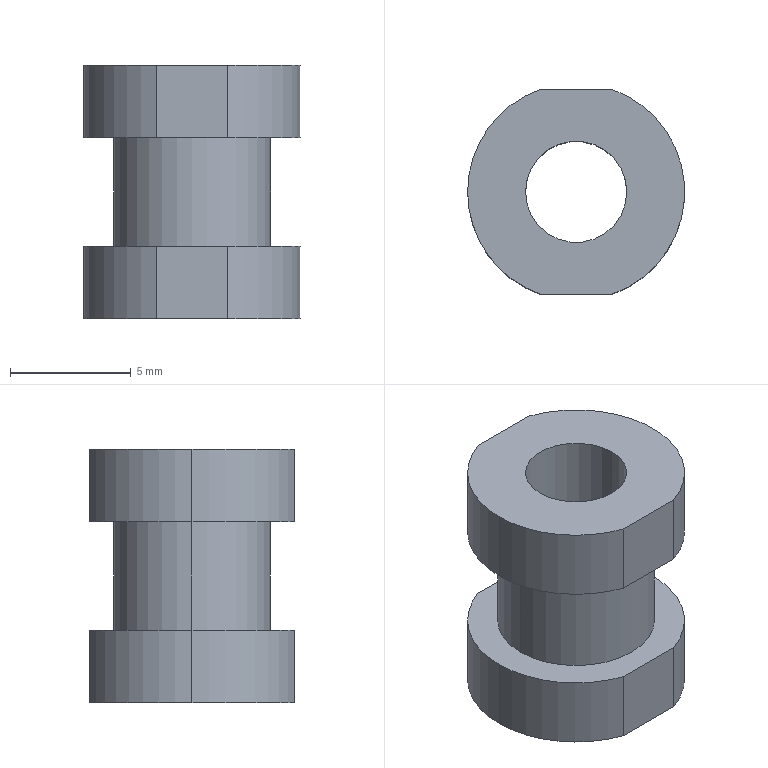Part | NX | features BREP 1 | 1 solid | 18 faces | box 9 x 8.5 x 10.5 mm | volume 379.606 mm3 | cylinder 10 | plane 8 | commonest cylinder face diameters 9 x6 4.2 x2 6.5 x2
STEP:
#1=CARTESIAN_POINT('',(9.871,10.94,0.));
#2=VERTEX_POINT('',#1);
#3=CARTESIAN_POINT('',(14.071,10.94,0.));
#4=VERTEX_POINT('',#3);
#5=CARTESIAN_POINT('',(11.971,10.94,0.));
#6=DIRECTION('',(0.,0.,1.));
#7=DIRECTION('',(1.,0.,0.));
#8=AXIS2_PLACEMENT_3D('',#5,#6,#7);
#9=CIRCLE('',#8,2.1);
#10=EDGE_CURVE('',#2,#4,#9,.T.);
#11=ORIENTED_EDGE('',*,*,#10,.F.);
#12=CARTESIAN_POINT('',(9.871,10.94,10.5));
#13=VERTEX_POINT('',#12);
#14=CARTESIAN_POINT('',(9.871,10.94,10.5));
#15=DIRECTION('',(0.,0.,1.));
#16=VECTOR('',#15,1000.);
#17=LINE('',#14,#16);
#18=EDGE_CURVE('',#13,#2,#17,.F.);
#19=ORIENTED_EDGE('',*,*,#18,.F.);
#20=CARTESIAN_POINT('',(14.071,10.94,10.5));
#21=VERTEX_POINT('',#20);
#22=CARTESIAN_POINT('',(11.971,10.94,10.5));
#23=DIRECTION('',(0.,0.,1.));
#24=DIRECTION('',(1.,0.,0.));
#25=AXIS2_PLACEMENT_3D('',#22,#23,#24);
#26=CIRCLE('',#25,2.1);
#27=EDGE_CURVE('',#13,#21,#26,.T.);
#28=ORIENTED_EDGE('',*,*,#27,.T.);
#29=CARTESIAN_POINT('',(14.071,10.94,10.5));
#30=DIRECTION('',(0.,0.,1.));
#31=VECTOR('',#30,1000.);
#32=LINE('',#29,#31);
#33=EDGE_CURVE('',#21,#4,#32,.F.);
#34=ORIENTED_EDGE('',*,*,#33,.T.);
#35=EDGE_LOOP('',(#11,#19,#28,#34));
#36=FACE_BOUND('',#35,.T.);
#37=CARTESIAN_POINT('',(11.971,10.94,10.5));
#38=DIRECTION('',(0.,0.,1.));
#39=DIRECTION('',(1.,0.,0.));
#40=AXIS2_PLACEMENT_3D('',#37,#38,#39);
#41=CYLINDRICAL_SURFACE('',#40,2.1);
#42=ADVANCED_FACE('',(#36),#41,.F.);
#43=CARTESIAN_POINT('',(15.221,10.94,7.5));
#44=VERTEX_POINT('',#43);
#45=CARTESIAN_POINT('',(8.721,10.94,7.5));
#46=VERTEX_POINT('',#45);
#47=CARTESIAN_POINT('',(11.971,10.94,7.5));
#48=DIRECTION('',(0.,0.,1.));
#49=DIRECTION('',(1.,0.,0.));
#50=AXIS2_PLACEMENT_3D('',#47,#48,#49);
#51=CIRCLE('',#50,3.25);
#52=EDGE_CURVE('',#44,#46,#51,.T.);
#53=ORIENTED_EDGE('',*,*,#52,.F.);
#54=CARTESIAN_POINT('',(15.221,10.94,3.));
#55=VERTEX_POINT('',#54);
#56=CARTESIAN_POINT('',(15.221,10.94,7.5));
#57=DIRECTION('',(0.,0.,-1.));
#58=VECTOR('',#57,1000.);
#59=LINE('',#56,#58);
#60=EDGE_CURVE('',#44,#55,#59,.T.);
#61=ORIENTED_EDGE('',*,*,#60,.T.);
#62=CARTESIAN_POINT('',(8.721,10.94,3.));
#63=VERTEX_POINT('',#62);
#64=CARTESIAN_POINT('',(11.971,10.94,3.));
#65=DIRECTION('',(0.,0.,1.));
#66=DIRECTION('',(1.,0.,0.));
#67=AXIS2_PLACEMENT_3D('',#64,#65,#66);
#68=CIRCLE('',#67,3.25);
#69=EDGE_CURVE('',#55,#63,#68,.T.);
#70=ORIENTED_EDGE('',*,*,#69,.T.);
#71=CARTESIAN_POINT('',(8.721,10.94,7.5));
#72=DIRECTION('',(0.,0.,-1.));
#73=VECTOR('',#72,1000.);
#74=LINE('',#71,#73);
#75=EDGE_CURVE('',#46,#63,#74,.T.);
#76=ORIENTED_EDGE('',*,*,#75,.F.);
#77=EDGE_LOOP('',(#53,#61,#70,#76));
#78=FACE_BOUND('',#77,.T.);
#79=CARTESIAN_POINT('',(11.971,10.94,7.5));
#80=DIRECTION('',(0.,0.,-1.));
#81=DIRECTION('',(-1.,0.,0.));
#82=AXIS2_PLACEMENT_3D('',#79,#80,#81);
#83=CYLINDRICAL_SURFACE('',#82,3.25);
#84=ADVANCED_FACE('',(#78),#83,.T.);
#85=CARTESIAN_POINT('',(7.471,10.94,10.5));
#86=VERTEX_POINT('',#85);
#87=CARTESIAN_POINT('',(10.492,6.69,10.5));
#88=VERTEX_POINT('',#87);
#89=CARTESIAN_POINT('',(11.971,10.94,10.5));
#90=DIRECTION('',(0.,0.,1.));
#91=DIRECTION('',(1.,0.,0.));
#92=AXIS2_PLACEMENT_3D('',#89,#90,#91);
#93=CIRCLE('',#92,4.5);
#94=EDGE_CURVE('',#86,#88,#93,.T.);
#95=ORIENTED_EDGE('',*,*,#94,.F.);
#96=CARTESIAN_POINT('',(7.471,10.94,7.5));
#97=VERTEX_POINT('',#96);
#98=CARTESIAN_POINT('',(7.471,10.94,10.5));
#99=DIRECTION('',(0.,0.,-1.));
#100=VECTOR('',#99,1000.);
#101=LINE('',#98,#100);
#102=EDGE_CURVE('',#86,#97,#101,.T.);
#103=ORIENTED_EDGE('',*,*,#102,.T.);
#104=CARTESIAN_POINT('',(10.492,6.69,7.5));
#105=VERTEX_POINT('',#104);
#106=CARTESIAN_POINT('',(11.971,10.94,7.5));
#107=DIRECTION('',(0.,0.,1.));
#108=DIRECTION('',(1.,0.,0.));
#109=AXIS2_PLACEMENT_3D('',#106,#107,#108);
#110=CIRCLE('',#109,4.5);
#111=EDGE_CURVE('',#97,#105,#110,.T.);
#112=ORIENTED_EDGE('',*,*,#111,.T.);
#113=CARTESIAN_POINT('',(10.492,6.69,10.5));
#114=DIRECTION('',(0.,0.,-1.));
#115=VECTOR('',#114,1000.);
#116=LINE('',#113,#115);
#117=EDGE_CURVE('',#88,#105,#116,.T.);
#118=ORIENTED_EDGE('',*,*,#117,.F.);
#119=EDGE_LOOP('',(#95,#103,#112,#118));
#120=FACE_BOUND('',#119,.T.);
#121=CARTESIAN_POINT('',(11.971,10.94,10.5));
#122=DIRECTION('',(0.,0.,-1.));
#123=DIRECTION('',(-1.,0.,0.));
#124=AXIS2_PLACEMENT_3D('',#121,#122,#123);
#125=CYLINDRICAL_SURFACE('',#124,4.5);
#126=ADVANCED_FACE('',(#120),#125,.T.);
#127=CARTESIAN_POINT('',(7.471,10.94,3.));
#128=VERTEX_POINT('',#127);
#129=CARTESIAN_POINT('',(10.492,6.69,3.));
#130=VERTEX_POINT('',#129);
#131=CARTESIAN_POINT('',(11.971,10.94,3.));
#132=DIRECTION('',(0.,0.,1.));
#133=DIRECTION('',(1.,0.,0.));
#134=AXIS2_PLACEMENT_3D('',#131,#132,#133);
#135=CIRCLE('',#134,4.5);
#136=EDGE_CURVE('',#128,#130,#135,.T.);
#137=ORIENTED_EDGE('',*,*,#136,.F.);
#138=CARTESIAN_POINT('',(7.471,10.94,0.));
#139=VERTEX_POINT('',#138);
#140=CARTESIAN_POINT('',(7.471,10.94,3.));
#141=DIRECTION('',(0.,0.,-1.));
#142=VECTOR('',#141,1000.);
#143=LINE('',#140,#142);
#144=EDGE_CURVE('',#128,#139,#143,.T.);
#145=ORIENTED_EDGE('',*,*,#144,.T.);
#146=CARTESIAN_POINT('',(10.492,6.69,0.));
#147=VERTEX_POINT('',#146);
#148=CARTESIAN_POINT('',(11.971,10.94,0.));
#149=DIRECTION('',(0.,0.,1.));
#150=DIRECTION('',(1.,0.,0.));
#151=AXIS2_PLACEMENT_3D('',#148,#149,#150);
#152=CIRCLE('',#151,4.5);
#153=EDGE_CURVE('',#139,#147,#152,.T.);
#154=ORIENTED_EDGE('',*,*,#153,.T.);
#155=CARTESIAN_POINT('',(10.492,6.69,3.));
#156=DIRECTION('',(0.,0.,-1.));
#157=VECTOR('',#156,1000.);
#158=LINE('',#155,#157);
#159=EDGE_CURVE('',#130,#147,#158,.T.);
#160=ORIENTED_EDGE('',*,*,#159,.F.);
#161=EDGE_LOOP('',(#137,#145,#154,#160));
#162=FACE_BOUND('',#161,.T.);
#163=CARTESIAN_POINT('',(11.971,10.94,3.));
#164=DIRECTION('',(0.,0.,-1.));
#165=DIRECTION('',(-1.,0.,0.));
#166=AXIS2_PLACEMENT_3D('',#163,#164,#165);
#167=CYLINDRICAL_SURFACE('',#166,4.5);
#168=ADVANCED_FACE('',(#162),#167,.T.);
#169=CARTESIAN_POINT('',(10.492,15.19,3.));
#170=VERTEX_POINT('',#169);
#171=CARTESIAN_POINT('',(11.971,10.94,3.));
#172=DIRECTION('',(0.,0.,1.));
#173=DIRECTION('',(1.,0.,0.));
#174=AXIS2_PLACEMENT_3D('',#171,#172,#173);
#175=CIRCLE('',#174,4.5);
#176=EDGE_CURVE('',#170,#128,#175,.T.);
#177=ORIENTED_EDGE('',*,*,#176,.T.);
#178=ORIENTED_EDGE('',*,*,#136,.T.);
#179=CARTESIAN_POINT('',(13.451,6.69,3.));
#180=VERTEX_POINT('',#179);
#181=CARTESIAN_POINT('',(11.971,6.69,3.));
#182=DIRECTION('',(1.,0.,0.));
#183=VECTOR('',#182,1000.);
#184=LINE('',#181,#183);
#185=EDGE_CURVE('',#130,#180,#184,.T.);
#186=ORIENTED_EDGE('',*,*,#185,.T.);
#187=CARTESIAN_POINT('',(13.451,15.19,3.));
#188=VERTEX_POINT('',#187);
#189=CARTESIAN_POINT('',(11.971,10.94,3.));
#190=DIRECTION('',(0.,0.,1.));
#191=DIRECTION('',(1.,0.,0.));
#192=AXIS2_PLACEMENT_3D('',#189,#190,#191);
#193=CIRCLE('',#192,4.5);
#194=EDGE_CURVE('',#180,#188,#193,.T.);
#195=ORIENTED_EDGE('',*,*,#194,.T.);
#196=CARTESIAN_POINT('',(11.971,15.19,3.));
#197=DIRECTION('',(-1.,0.,0.));
#198=VECTOR('',#197,1000.);
#199=LINE('',#196,#198);
#200=EDGE_CURVE('',#188,#170,#199,.T.);
#201=ORIENTED_EDGE('',*,*,#200,.T.);
#202=EDGE_LOOP('',(#177,#178,#186,#195,#201));
#203=FACE_BOUND('',#202,.T.);
#204=CARTESIAN_POINT('',(11.971,10.94,3.));
#205=DIRECTION('',(0.,0.,1.));
#206=DIRECTION('',(1.,0.,0.));
#207=AXIS2_PLACEMENT_3D('',#204,#205,#206);
#208=CIRCLE('',#207,3.25);
#209=EDGE_CURVE('',#63,#55,#208,.T.);
#210=ORIENTED_EDGE('',*,*,#209,.F.);
#211=ORIENTED_EDGE('',*,*,#69,.F.);
#212=EDGE_LOOP('',(#210,#211));
#213=FACE_BOUND('',#212,.T.);
#214=CARTESIAN_POINT('',(11.971,10.94,3.));
#215=DIRECTION('',(0.,0.,1.));
#216=DIRECTION('',(1.,0.,0.));
#217=AXIS2_PLACEMENT_3D('',#214,#215,#216);
#218=PLANE('',#217);
#219=ADVANCED_FACE('',(#203,#213),#218,.T.);
#220=ORIENTED_EDGE('',*,*,#144,.F.);
#221=ORIENTED_EDGE('',*,*,#176,.F.);
#222=CARTESIAN_POINT('',(10.492,15.19,0.));
#223=VERTEX_POINT('',#222);
#224=CARTESIAN_POINT('',(10.492,15.19,3.));
#225=DIRECTION('',(0.,0.,1.));
#226=VECTOR('',#225,1000.);
#227=LINE('',#224,#226);
#228=EDGE_CURVE('',#223,#170,#227,.T.);
#229=ORIENTED_EDGE('',*,*,#228,.F.);
#230=CARTESIAN_POINT('',(11.971,10.94,0.));
#231=DIRECTION('',(0.,0.,1.));
#232=DIRECTION('',(1.,0.,0.));
#233=AXIS2_PLACEMENT_3D('',#230,#231,#232);
#234=CIRCLE('',#233,4.5);
#235=EDGE_CURVE('',#223,#139,#234,.T.);
#236=ORIENTED_EDGE('',*,*,#235,.T.);
#237=EDGE_LOOP('',(#220,#221,#229,#236));
#238=FACE_BOUND('',#237,.T.);
#239=CARTESIAN_POINT('',(11.971,10.94,3.));
#240=DIRECTION('',(0.,0.,-1.));
#241=DIRECTION('',(-1.,0.,0.));
#242=AXIS2_PLACEMENT_3D('',#239,#240,#241);
#243=CYLINDRICAL_SURFACE('',#242,4.5);
#244=ADVANCED_FACE('',(#238),#243,.T.);
#245=CARTESIAN_POINT('',(13.451,6.69,0.));
#246=VERTEX_POINT('',#245);
#247=CARTESIAN_POINT('',(13.451,6.69,3.));
#248=DIRECTION('',(0.,0.,1.));
#249=VECTOR('',#248,1000.);
#250=LINE('',#247,#249);
#251=EDGE_CURVE('',#246,#180,#250,.T.);
#252=ORIENTED_EDGE('',*,*,#251,.F.);
#253=CARTESIAN_POINT('',(13.451,15.19,0.));
#254=VERTEX_POINT('',#253);
#255=CARTESIAN_POINT('',(11.971,10.94,0.));
#256=DIRECTION('',(0.,0.,1.));
#257=DIRECTION('',(1.,0.,0.));
#258=AXIS2_PLACEMENT_3D('',#255,#256,#257);
#259=CIRCLE('',#258,4.5);
#260=EDGE_CURVE('',#246,#254,#259,.T.);
#261=ORIENTED_EDGE('',*,*,#260,.T.);
#262=CARTESIAN_POINT('',(13.451,15.19,3.));
#263=DIRECTION('',(0.,0.,-1.));
#264=VECTOR('',#263,1000.);
#265=LINE('',#262,#264);
#266=EDGE_CURVE('',#188,#254,#265,.T.);
#267=ORIENTED_EDGE('',*,*,#266,.F.);
#268=ORIENTED_EDGE('',*,*,#194,.F.);
#269=EDGE_LOOP('',(#252,#261,#267,#268));
#270=FACE_BOUND('',#269,.T.);
#271=CARTESIAN_POINT('',(11.971,10.94,3.));
#272=DIRECTION('',(0.,0.,-1.));
#273=DIRECTION('',(-1.,0.,0.));
#274=AXIS2_PLACEMENT_3D('',#271,#272,#273);
#275=CYLINDRICAL_SURFACE('',#274,4.5);
#276=ADVANCED_FACE('',(#270),#275,.T.);
#277=CARTESIAN_POINT('',(0.2618,6.69,0.));
#278=DIRECTION('',(1.,0.,0.));
#279=VECTOR('',#278,1000.);
#280=LINE('',#277,#279);
#281=EDGE_CURVE('',#147,#246,#280,.T.);
#282=ORIENTED_EDGE('',*,*,#281,.F.);
#283=ORIENTED_EDGE('',*,*,#153,.F.);
#284=ORIENTED_EDGE('',*,*,#235,.F.);
#285=CARTESIAN_POINT('',(0.2618,15.19,0.));
#286=DIRECTION('',(-1.,0.,0.));
#287=VECTOR('',#286,1000.);
#288=LINE('',#285,#287);
#289=EDGE_CURVE('',#254,#223,#288,.T.);
#290=ORIENTED_EDGE('',*,*,#289,.F.);
#291=ORIENTED_EDGE('',*,*,#260,.F.);
#292=EDGE_LOOP('',(#282,#283,#284,#290,#291));
#293=FACE_BOUND('',#292,.T.);
#294=CARTESIAN_POINT('',(11.971,10.94,0.));
#295=DIRECTION('',(0.,0.,1.));
#296=DIRECTION('',(1.,0.,0.));
#297=AXIS2_PLACEMENT_3D('',#294,#295,#296);
#298=CIRCLE('',#297,2.1);
#299=EDGE_CURVE('',#4,#2,#298,.T.);
#300=ORIENTED_EDGE('',*,*,#299,.T.);
#301=ORIENTED_EDGE('',*,*,#10,.T.);
#302=EDGE_LOOP('',(#300,#301));
#303=FACE_BOUND('',#302,.T.);
#304=CARTESIAN_POINT('',(11.971,10.94,0.));
#305=DIRECTION('',(0.,0.,1.));
#306=DIRECTION('',(1.,0.,0.));
#307=AXIS2_PLACEMENT_3D('',#304,#305,#306);
#308=PLANE('',#307);
#309=ADVANCED_FACE('',(#293,#303),#308,.F.);
#310=CARTESIAN_POINT('',(13.451,6.69,7.5));
#311=VERTEX_POINT('',#310);
#312=CARTESIAN_POINT('',(11.971,6.69,7.5));
#313=DIRECTION('',(1.,0.,0.));
#314=VECTOR('',#313,1000.);
#315=LINE('',#312,#314);
#316=EDGE_CURVE('',#105,#311,#315,.T.);
#317=ORIENTED_EDGE('',*,*,#316,.F.);
#318=ORIENTED_EDGE('',*,*,#111,.F.);
#319=CARTESIAN_POINT('',(10.492,15.19,7.5));
#320=VERTEX_POINT('',#319);
#321=CARTESIAN_POINT('',(11.971,10.94,7.5));
#322=DIRECTION('',(0.,0.,1.));
#323=DIRECTION('',(1.,0.,0.));
#324=AXIS2_PLACEMENT_3D('',#321,#322,#323);
#325=CIRCLE('',#324,4.5);
#326=EDGE_CURVE('',#320,#97,#325,.T.);
#327=ORIENTED_EDGE('',*,*,#326,.F.);
#328=CARTESIAN_POINT('',(13.451,15.19,7.5));
#329=VERTEX_POINT('',#328);
#330=CARTESIAN_POINT('',(11.971,15.19,7.5));
#331=DIRECTION('',(-1.,0.,0.));
#332=VECTOR('',#331,1000.);
#333=LINE('',#330,#332);
#334=EDGE_CURVE('',#329,#320,#333,.T.);
#335=ORIENTED_EDGE('',*,*,#334,.F.);
#336=CARTESIAN_POINT('',(11.971,10.94,7.5));
#337=DIRECTION('',(0.,0.,1.));
#338=DIRECTION('',(1.,0.,0.));
#339=AXIS2_PLACEMENT_3D('',#336,#337,#338);
#340=CIRCLE('',#339,4.5);
#341=EDGE_CURVE('',#311,#329,#340,.T.);
#342=ORIENTED_EDGE('',*,*,#341,.F.);
#343=EDGE_LOOP('',(#317,#318,#327,#335,#342));
#344=FACE_BOUND('',#343,.T.);
#345=CARTESIAN_POINT('',(11.971,10.94,7.5));
#346=DIRECTION('',(0.,0.,1.));
#347=DIRECTION('',(1.,0.,0.));
#348=AXIS2_PLACEMENT_3D('',#345,#346,#347);
#349=CIRCLE('',#348,3.25);
#350=EDGE_CURVE('',#46,#44,#349,.T.);
#351=ORIENTED_EDGE('',*,*,#350,.T.);
#352=ORIENTED_EDGE('',*,*,#52,.T.);
#353=EDGE_LOOP('',(#351,#352));
#354=FACE_BOUND('',#353,.T.);
#355=CARTESIAN_POINT('',(11.971,10.94,7.5));
#356=DIRECTION('',(0.,0.,1.));
#357=DIRECTION('',(1.,0.,0.));
#358=AXIS2_PLACEMENT_3D('',#355,#356,#357);
#359=PLANE('',#358);
#360=ADVANCED_FACE('',(#344,#354),#359,.F.);
#361=ORIENTED_EDGE('',*,*,#102,.F.);
#362=CARTESIAN_POINT('',(10.492,15.19,10.5));
#363=VERTEX_POINT('',#362);
#364=CARTESIAN_POINT('',(11.971,10.94,10.5));
#365=DIRECTION('',(0.,0.,1.));
#366=DIRECTION('',(1.,0.,0.));
#367=AXIS2_PLACEMENT_3D('',#364,#365,#366);
#368=CIRCLE('',#367,4.5);
#369=EDGE_CURVE('',#363,#86,#368,.T.);
#370=ORIENTED_EDGE('',*,*,#369,.F.);
#371=CARTESIAN_POINT('',(10.492,15.19,10.5));
#372=DIRECTION('',(0.,0.,1.));
#373=VECTOR('',#372,1000.);
#374=LINE('',#371,#373);
#375=EDGE_CURVE('',#320,#363,#374,.T.);
#376=ORIENTED_EDGE('',*,*,#375,.F.);
#377=ORIENTED_EDGE('',*,*,#326,.T.);
#378=EDGE_LOOP('',(#361,#370,#376,#377));
#379=FACE_BOUND('',#378,.T.);
#380=CARTESIAN_POINT('',(11.971,10.94,10.5));
#381=DIRECTION('',(0.,0.,-1.));
#382=DIRECTION('',(-1.,0.,0.));
#383=AXIS2_PLACEMENT_3D('',#380,#381,#382);
#384=CYLINDRICAL_SURFACE('',#383,4.5);
#385=ADVANCED_FACE('',(#379),#384,.T.);
#386=CARTESIAN_POINT('',(13.451,6.69,10.5));
#387=VERTEX_POINT('',#386);
#388=CARTESIAN_POINT('',(13.451,6.69,10.5));
#389=DIRECTION('',(0.,0.,1.));
#390=VECTOR('',#389,1000.);
#391=LINE('',#388,#390);
#392=EDGE_CURVE('',#311,#387,#391,.T.);
#393=ORIENTED_EDGE('',*,*,#392,.F.);
#394=ORIENTED_EDGE('',*,*,#341,.T.);
#395=CARTESIAN_POINT('',(13.451,15.19,10.5));
#396=VERTEX_POINT('',#395);
#397=CARTESIAN_POINT('',(13.451,15.19,10.5));
#398=DIRECTION('',(0.,0.,-1.));
#399=VECTOR('',#398,1000.);
#400=LINE('',#397,#399);
#401=EDGE_CURVE('',#396,#329,#400,.T.);
#402=ORIENTED_EDGE('',*,*,#401,.F.);
#403=CARTESIAN_POINT('',(11.971,10.94,10.5));
#404=DIRECTION('',(0.,0.,1.));
#405=DIRECTION('',(1.,0.,0.));
#406=AXIS2_PLACEMENT_3D('',#403,#404,#405);
#407=CIRCLE('',#406,4.5);
#408=EDGE_CURVE('',#387,#396,#407,.T.);
#409=ORIENTED_EDGE('',*,*,#408,.F.);
#410=EDGE_LOOP('',(#393,#394,#402,#409));
#411=FACE_BOUND('',#410,.T.);
#412=CARTESIAN_POINT('',(11.971,10.94,10.5));
#413=DIRECTION('',(0.,0.,-1.));
#414=DIRECTION('',(-1.,0.,0.));
#415=AXIS2_PLACEMENT_3D('',#412,#413,#414);
#416=CYLINDRICAL_SURFACE('',#415,4.5);
#417=ADVANCED_FACE('',(#411),#416,.T.);
#418=ORIENTED_EDGE('',*,*,#369,.T.);
#419=ORIENTED_EDGE('',*,*,#94,.T.);
#420=CARTESIAN_POINT('',(11.971,6.69,10.5));
#421=DIRECTION('',(1.,0.,0.));
#422=VECTOR('',#421,1000.);
#423=LINE('',#420,#422);
#424=EDGE_CURVE('',#88,#387,#423,.T.);
#425=ORIENTED_EDGE('',*,*,#424,.T.);
#426=ORIENTED_EDGE('',*,*,#408,.T.);
#427=CARTESIAN_POINT('',(11.971,15.19,10.5));
#428=DIRECTION('',(-1.,0.,0.));
#429=VECTOR('',#428,1000.);
#430=LINE('',#427,#429);
#431=EDGE_CURVE('',#396,#363,#430,.T.);
#432=ORIENTED_EDGE('',*,*,#431,.T.);
#433=EDGE_LOOP('',(#418,#419,#425,#426,#432));
#434=FACE_BOUND('',#433,.T.);
#435=CARTESIAN_POINT('',(11.971,10.94,10.5));
#436=DIRECTION('',(0.,0.,1.));
#437=DIRECTION('',(1.,0.,0.));
#438=AXIS2_PLACEMENT_3D('',#435,#436,#437);
#439=CIRCLE('',#438,2.1);
#440=EDGE_CURVE('',#21,#13,#439,.T.);
#441=ORIENTED_EDGE('',*,*,#440,.F.);
#442=ORIENTED_EDGE('',*,*,#27,.F.);
#443=EDGE_LOOP('',(#441,#442));
#444=FACE_BOUND('',#443,.T.);
#445=CARTESIAN_POINT('',(11.971,10.94,10.5));
#446=DIRECTION('',(0.,0.,1.));
#447=DIRECTION('',(1.,0.,0.));
#448=AXIS2_PLACEMENT_3D('',#445,#446,#447);
#449=PLANE('',#448);
#450=ADVANCED_FACE('',(#434,#444),#449,.T.);
#451=ORIENTED_EDGE('',*,*,#60,.F.);
#452=ORIENTED_EDGE('',*,*,#350,.F.);
#453=ORIENTED_EDGE('',*,*,#75,.T.);
#454=ORIENTED_EDGE('',*,*,#209,.T.);
#455=EDGE_LOOP('',(#451,#452,#453,#454));
#456=FACE_BOUND('',#455,.T.);
#457=CARTESIAN_POINT('',(11.971,10.94,7.5));
#458=DIRECTION('',(0.,0.,-1.));
#459=DIRECTION('',(-1.,0.,0.));
#460=AXIS2_PLACEMENT_3D('',#457,#458,#459);
#461=CYLINDRICAL_SURFACE('',#460,3.25);
#462=ADVANCED_FACE('',(#456),#461,.T.);
#463=ORIENTED_EDGE('',*,*,#18,.T.);
#464=ORIENTED_EDGE('',*,*,#299,.F.);
#465=ORIENTED_EDGE('',*,*,#33,.F.);
#466=ORIENTED_EDGE('',*,*,#440,.T.);
#467=EDGE_LOOP('',(#463,#464,#465,#466));
#468=FACE_BOUND('',#467,.T.);
#469=CARTESIAN_POINT('',(11.971,10.94,10.5));
#470=DIRECTION('',(0.,0.,1.));
#471=DIRECTION('',(1.,0.,0.));
#472=AXIS2_PLACEMENT_3D('',#469,#470,#471);
#473=CYLINDRICAL_SURFACE('',#472,2.1);
#474=ADVANCED_FACE('',(#468),#473,.F.);
#475=ORIENTED_EDGE('',*,*,#401,.T.);
#476=ORIENTED_EDGE('',*,*,#334,.T.);
#477=ORIENTED_EDGE('',*,*,#375,.T.);
#478=ORIENTED_EDGE('',*,*,#431,.F.);
#479=EDGE_LOOP('',(#475,#476,#477,#478));
#480=FACE_BOUND('',#479,.T.);
#481=CARTESIAN_POINT('',(0.2618,15.19,0.));
#482=DIRECTION('',(0.,1.,0.));
#483=DIRECTION('',(1.,0.,0.));
#484=AXIS2_PLACEMENT_3D('',#481,#482,#483);
#485=PLANE('',#484);
#486=ADVANCED_FACE('',(#480),#485,.T.);
#487=ORIENTED_EDGE('',*,*,#117,.T.);
#488=ORIENTED_EDGE('',*,*,#316,.T.);
#489=ORIENTED_EDGE('',*,*,#392,.T.);
#490=ORIENTED_EDGE('',*,*,#424,.F.);
#491=EDGE_LOOP('',(#487,#488,#489,#490));
#492=FACE_BOUND('',#491,.T.);
#493=CARTESIAN_POINT('',(0.2618,6.69,0.));
#494=DIRECTION('',(0.,-1.,0.));
#495=DIRECTION('',(0.,0.,-1.));
#496=AXIS2_PLACEMENT_3D('',#493,#494,#495);
#497=PLANE('',#496);
#498=ADVANCED_FACE('',(#492),#497,.T.);
#499=ORIENTED_EDGE('',*,*,#266,.T.);
#500=ORIENTED_EDGE('',*,*,#289,.T.);
#501=ORIENTED_EDGE('',*,*,#228,.T.);
#502=ORIENTED_EDGE('',*,*,#200,.F.);
#503=EDGE_LOOP('',(#499,#500,#501,#502));
#504=FACE_BOUND('',#503,.T.);
#505=CARTESIAN_POINT('',(0.2618,15.19,0.));
#506=DIRECTION('',(0.,1.,0.));
#507=DIRECTION('',(1.,0.,0.));
#508=AXIS2_PLACEMENT_3D('',#505,#506,#507);
#509=PLANE('',#508);
#510=ADVANCED_FACE('',(#504),#509,.T.);
#511=ORIENTED_EDGE('',*,*,#159,.T.);
#512=ORIENTED_EDGE('',*,*,#281,.T.);
#513=ORIENTED_EDGE('',*,*,#251,.T.);
#514=ORIENTED_EDGE('',*,*,#185,.F.);
#515=EDGE_LOOP('',(#511,#512,#513,#514));
#516=FACE_BOUND('',#515,.T.);
#517=CARTESIAN_POINT('',(0.2618,6.69,0.));
#518=DIRECTION('',(0.,-1.,0.));
#519=DIRECTION('',(0.,0.,-1.));
#520=AXIS2_PLACEMENT_3D('',#517,#518,#519);
#521=PLANE('',#520);
#522=ADVANCED_FACE('',(#516),#521,.T.);
#523=CLOSED_SHELL('',(#42,#84,#126,#168,#219,#244,#276,#309,#360,#385,#417,#450,#462,#474,#486,#498,#510,#522));
#524=MANIFOLD_SOLID_BREP('',#523);
#525=(LENGTH_UNIT()NAMED_UNIT(*)SI_UNIT(.MILLI.,.METRE.));
#526=UNCERTAINTY_MEASURE_WITH_UNIT(LENGTH_MEASURE(0.00001),#525,'','');
#527=(NAMED_UNIT(*)PLANE_ANGLE_UNIT()SI_UNIT($,.RADIAN.));
#528=(NAMED_UNIT(*)SI_UNIT($,.STERADIAN.)SOLID_ANGLE_UNIT());
#529=(GEOMETRIC_REPRESENTATION_CONTEXT(3)GLOBAL_UNCERTAINTY_ASSIGNED_CONTEXT((#526))GLOBAL_UNIT_ASSIGNED_CONTEXT((#525,#527,#528))REPRESENTATION_CONTEXT('',''));
#530=ADVANCED_BREP_SHAPE_REPRESENTATION('',(#524),#529);